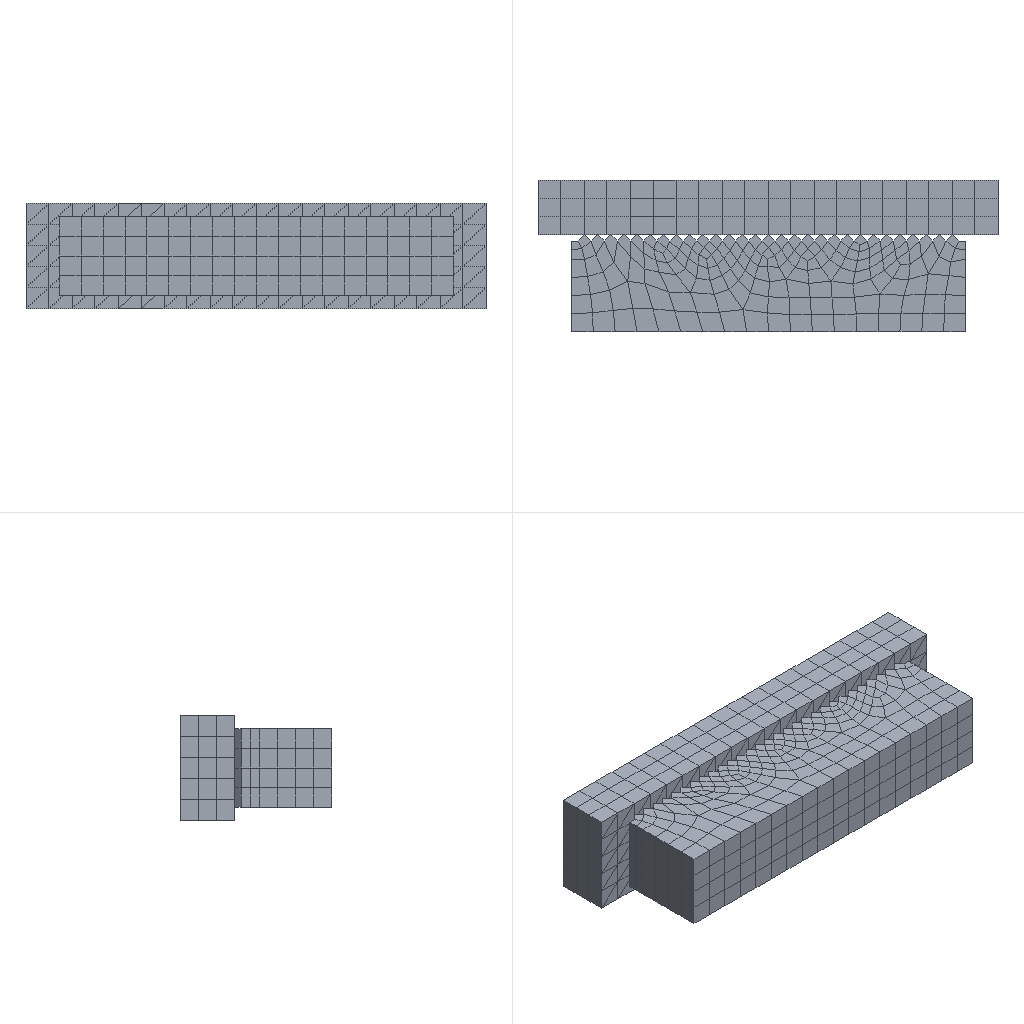Simulation study | ansys workbench
Ansys APDL input file, long lists of numbers shortened:
/batch
/config,noeldb,1     ! force off writing results to database
*get,_wallstrt,active,,time,wall
! ANSYS input file written by Workbench version 2022 R1
! File used for geometry attach: F:\ansys（分析文件汇总)\胶桶有限元分析\胶筒.STEP
/title,wbnew--____ (A5)
! ****** Begin Custom Load Command Snippet ******
/COM, ACT Extensions:
/COM,     LSDYNA, 2021.1
/COM,
! ****** End   Custom Load Command Snippet ******
*DIM,_wb_ProjectScratch_dir,string,248
_wb_ProjectScratch_dir(1) = 'C:\Users\Administrator\AppData\Local\Temp\WB_Administrator_5428_2\_ProjectScratch\Scr709D\'
*DIM,_wb_SolverFiles_dir,string,248
_wb_SolverFiles_dir(1) = 'C:\Users\Administrator\AppData\Local\Temp\WB_Administrator_5428_2\wbnew_files\dp0\SYS\MECH\'
*DIM,_wb_userfiles_dir,string,248
_wb_userfiles_dir(1) = 'C:\Users\Administrator\AppData\Local\Temp\WB_Administrator_5428_2\wbnew_files\user_files\'
/com,--- Data in consistent NMM units. See Solving Units in the help system for more information.
/units,MPA
/nopr
/wb,file,start              !  signify a WB generated input file
/prep7
! Turn off shape checking because checks already performed inside WB mesher.
! See help system for more information.
SHPP,OFF,,NOWARN
/nolist
etcon,set             ! allow ANSYS to choose best KEYOP's for 180x elements, resets any applicable keyopt to MAPDL defaults
/com,*********** Nodes for the whole assembly ***********
nblock,3,,6695
(1i9,3e20.9e3)
        1     2.926830022E+00    -1.817595946E+01    -1.336342308E+01
! (6086 more lines like these left out)
-1
/com,*********** Nodes for all Remote Points ***********
nblock,3
(1i9,3e20.9e3)
     6088     3.500000001E+01     4.276608832E-03    -8.325748840E-05
-1
/wb,elem,start            !  set before creation of elements
/com,*********** Elements for Body 1 "__-FreeParts|____1" ***********
et,1,186
keyo,1,2,1          ! set full integration on SOLID186
eblock,19,solid,,1098
(19i9)
        1        1        1        1        0        0        0        0       20        0        1        1        8       32        9      612      605      581      604
! (2195 more lines like these left out)
-1
/wb,elem,end               !  done creating elements
/com,*********** Send User Defined Coordinate System(s) ***********
csys,0
toffst,273.15,  ! Temperature offset from absolute zero
/com,*********** Set Reference Temperature ***********
tref,22.
/wb,mat,start              !  starting to send materials
/com,*********** Send Materials ***********
Temperature = 'TEMP' ! Temperature
MP,DENS,1,7.85e-09,	! tonne mm^-3
MP,ALPX,1,1.2e-05,	! C^-1
MP,C,1,434000000,	! mm^2 s^-2 C^-1
MP,KXX,1,60.5,	! tonne mm s^-3 C^-1
MP,RSVX,1,0.00017,	! ohm mm
MP,EX,1,200000,	! tonne s^-2 mm^-1
MP,NUXY,1,0.3,
MP,MURX,1,10000,
/wb,mat,end                !  done sending materials
!************************* Model Summary ********************
!__-FreeParts|____1,	结构钢,	matid,	1
!************************* End Model Summary ********************
! get the diagonal of the bounding box. Needed later for other things
*get,_xmin,node,,mnloc,x
*get,_ymin,node,,mnloc,y
*get,_zmin,node,,mnloc,z
*get,_xmax,node,,mxloc,x
*get,_ymax,node,,mxloc,y
*get,_zmax,node,,mxloc,z
_ASMDIAG=(_xmax-_xmin)*(_xmax-_xmin)+(_ymax-_ymin)*(_ymax-_ymin)+(_zmax-_zmin)*(_zmax-_zmin)
_ASMDIAG=SQRT(_ASMDIAG)
/wb,contact,start          !  starting to send contact
/wb,contact,end            !  done creating contacts
/golist
/wb,load,start             !  starting to send loads
/com,*********** Fixed Supports ***********
CMBLOCK,_FIXEDSU,NODE,      474
(8i10)
       579       580       581       582       583       584       585       586
! (59 more lines like these left out)
cmsel,s,_FIXEDSU
d,all,all
nsel,all
/com,*********** Create Remote Point "内部远程点" ***********
! -------- Remote Point Used by "力矩" --------
*set,tid,3
*set,cid,2
et,cid,174
et,tid,170
keyo,tid,2,1               ! Don't fix the pilot node
keyo,tid,4,111111
keyo,cid,12,5              ! Bonded Contact
keyo,cid,4,1               ! Deformable RBE3 style load
keyo,cid,2,2               ! MPC style contact
eblock,10,,,320
(15i9)
     2194        2        2        2        0     1206     1189     1174     1173     5197     5168     5164     5165
! (319 more lines like these left out)
-1
*set,_npilot,6088
_npilot32=_npilot
type,tid
mat ,cid
real,cid
tshape,pilo
en,2514,_npilot
tshape
/com,*********** Construct Moment Using Remote Attachment ***********
/gst,on,on
fini
*get,_numnode,node,0,count
*get,_numelem,elem,0,count
*get, _MAXELEMNUM, elem, 0, NUM, MAX
*get, _MAXNODENUM, node, 0, NUM, MAX
*get, _MAXELEMTYPE, etyp, 0, NUM, MAX
*get, _MAXREALCONST, real, 0, NUM, MAX
/go
/wb,load,end               !  done creating loads
/com,--- Number of total nodes = %_numnode%
/com,--- Number of contact elements = 320
/com,--- Number of spring elements = 0
/com,--- Number of bearing elements = 0
/com,--- Number of solid elements = 1098
/com,--- Number of condensed parts = 0
/com,--- Number of total elements = %_numelem%
*get,_wallbsol,active,,time,wall
/com,****************************************************************************
/com,*************************    SOLUTION       ********************************
/com,****************************************************************************
/solu
antype,0                   ! static analysis
_thickRatio=  1     ! Ratio of thick parts in the model
eqsl,pcg,1e-8,,,,,,1
cntr,print,1               ! print out contact info and also make no initial contact an error
dmpoption,emat,no             ! Don't combine emat file for DANSYS
dmpoption,esav,no             ! Don't combine esav file for DANSYS
nldiag,cont,iter           ! print out contact info each equilibrium iteration
rescontrol,,none                 ! Do not keep any restart files
/com,****************************************************
/com,******************* SOLVE FOR LS 1 OF 1 ****************
nsel,s,node,,6088
f,all,mx,500.
f,all,my,0.
f,all,mz,0.
nsel,all
/nopr
/gopr
nsub,1,1,1
time,1.
outres,erase
outres,all,none
outres,nsol,all,
outres,rsol,all
outres,eangl,all
outres,etmp,all
outres,veng,all
outres,strs,all,
outres,epel,all,
outres,eppl,all,
outres,cont,all,
! *********** WB SOLVE COMMAND ***********
! check interactive state
*get,ANSINTER_,active,,int
*if,ANSINTER_,ne,0,then
/eof
*endif
solve
/com *************** Write FE CONNECTORS *********
CEWRITE,file,ce,,INTE
/com,****************************************************
/com,*************** FINISHED SOLVE FOR LS 1 *************
*get,_wallasol,active,,time,wall
/nopr
*get,_numnode,node,0,count
*get,_numelem,elem,0,count
*get, _MAXELEMNUM, elem, 0, NUM, MAX
*get, _MAXNODENUM, node, 0, NUM, MAX,,,INTERNAL
*get, _MAXELEMTYPE, etyp, 0, NUM, MAX
*get, _MAXREALCONST, real, 0, NUM, MAX
/gopr
*get,_PCGITER,active,,solu,cgiter
/post1
xmlo,ENCODING,ISO-8859-1
xmlo,parm
/xml,parm,xml
fini
/gopr
*get,_walldone,active,,time,wall
_preptime=(_wallbsol-_wallstrt)*3600
_solvtime=(_wallasol-_wallbsol)*3600
_posttime=(_walldone-_wallasol)*3600
_totaltim=(_walldone-_wallstrt)*3600
*get,_dlbratio,active,0,solu,dlbr
*get,_combtime,active,0,solu,comb
*get,_ssmode,active,0,solu,ssmm
*get,_ndofs,active,0,solu,ndof
*get,_sol_end_time,active,0,set,time
*if,_sol_end_time,eq,1.,then
/fclean				!clean distributed files
*endif
/com,--- Total number of nodes = %_numnode%
/com,--- Total number of elements = %_numelem%
/com,--- Element load balance ratio = %_dlbratio%
/com,--- Time to combine distributed files = %_combtime%
/com,--- Sparse memory mode = %_ssmode%
/com,--- Number of DOF = %_ndofs%
/wb,file,end               ! done with WB generated input